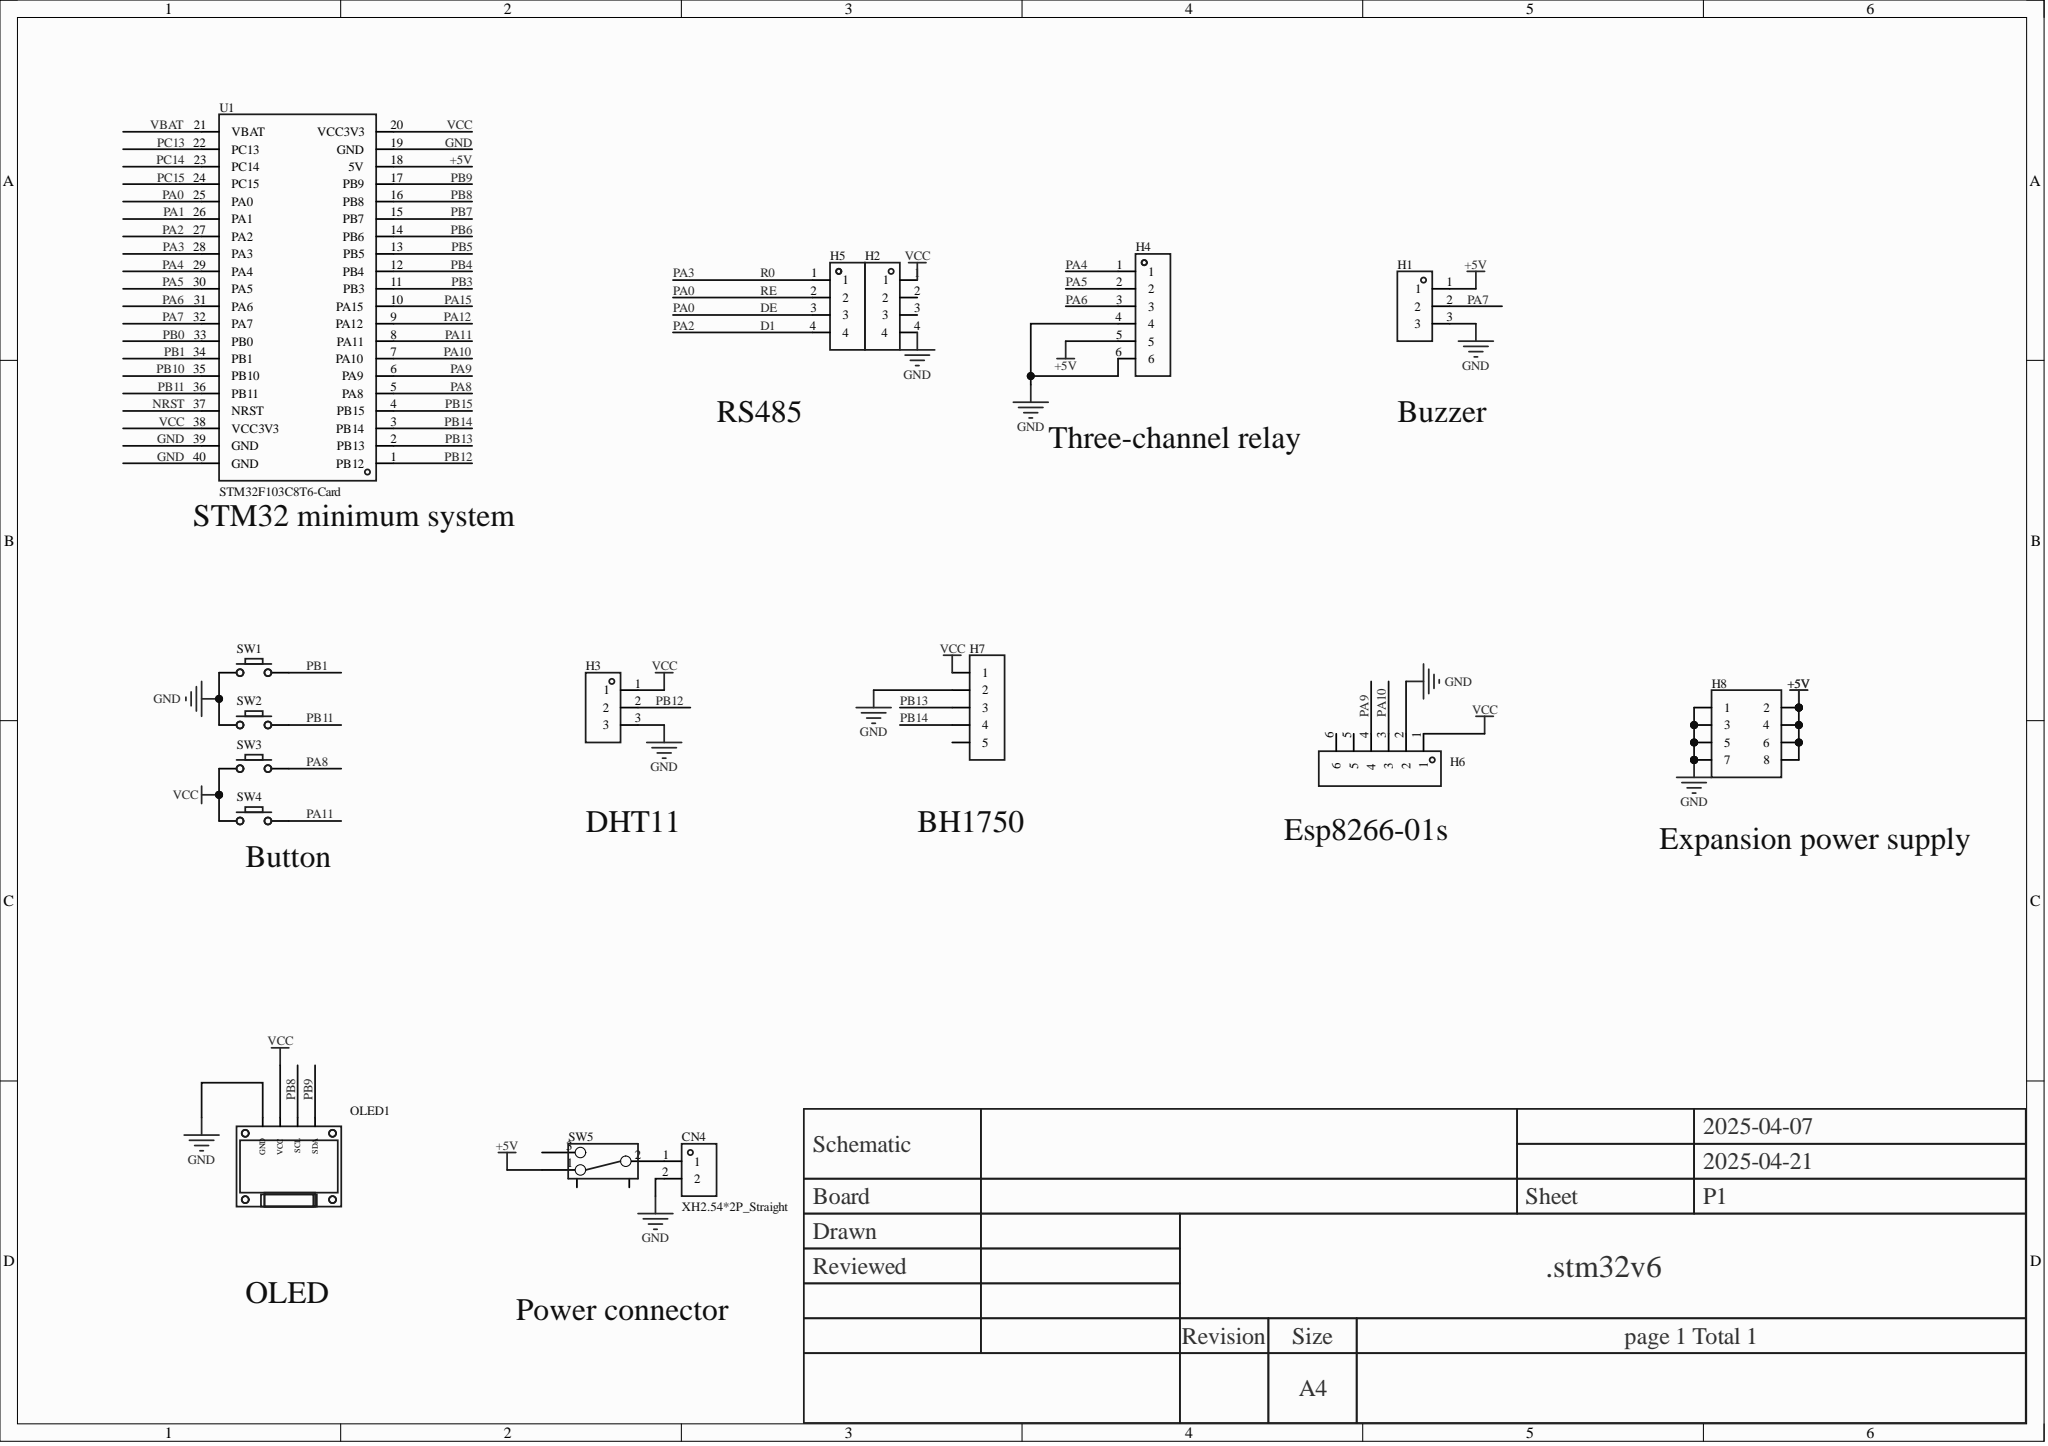Circuit board | Altium Designer | 16 parts | 22 nets
Bill of materials:
Comment,Description,Designator,Footprint,LibRef,Quantity
"XH2.54*2P_Straight","","CN4","CONN-TH_2P-P2.50-XH2.54-2P","XH2.54*2P_直插","1"
"","","H1, H3","HDR-TH_3P-P2.54-V-F","HDR-F_2.54_1x3P","2"
"","","H2, H5","HDR-TH_4P-P2.54-V-F","HDR-F_2.54_1x4P","2"
"","","H4, H6","HDR-TH_6P-P2.54-V-F","HDR-F_2.54_1x6P","2"
"","","H7","HDR-TH_5P-P2.54-V-F","HDR-F_2.54_1x5P","1"
"","","H8","HDR-TH_8P-P2.54-V-F-R2-C4-S2.54-1","HDR-F_2.54_2x4","1"
"","","OLED1","0.96OLED_4P","0.96OLED模块_4P","1"
"","","SW1, SW2, SW3, SW4","Key_TH_3.5x6x4.3","Key_TH_3.5x6x4.3","4"
"","","SW5","拨动开关","拨动开关_正","1"
"STM32F103C8T6-Card","","U1","CONN-TH_L53.3-W22.9_STM32F103C8T6-CARD","STM32F103C8T6-Card","1"
Netlist (Protel format):
[
CN4
CONN-TH_2P-P2.50-XH2.54-2P
XH2.54*2P_Straight



]
[
H1
HDR-TH_3P-P2.54-V-F




]
[
H2
HDR-TH_4P-P2.54-V-F




]
[
H3
HDR-TH_3P-P2.54-V-F




]
[
H4
HDR-TH_6P-P2.54-V-F




]
[
H5
HDR-TH_4P-P2.54-V-F




]
[
H6
HDR-TH_6P-P2.54-V-F




]
[
H7
HDR-TH_5P-P2.54-V-F




]
[
H8
HDR-TH_8P-P2.54-V-F-R2-C4-S2.54-1




]
[
OLED1
0.96OLED_4P




]
[
SW1
Key_TH_3.5x6x4.3




]
[
SW2
Key_TH_3.5x6x4.3




]
[
SW3
Key_TH_3.5x6x4.3




]
[
SW4
Key_TH_3.5x6x4.3




]
[
SW5
拨动开关




]
[
U1
CONN-TH_L53.3-W22.9_STM32F103C8T6-CARD
STM32F103C8T6-Card



]
(
VCC
H2-1
H3-1
H6-1
H7-1
OLED1-2
SW3-A
SW4-A
U1-20
U1-38
)
(
PB14
H7-4
U1-3
)
(
PB13
H7-3
U1-2
)
(
PB12
H3-2
U1-1
)
(
PB11
SW2-B
U1-36
)
(
PB9
OLED1-4
U1-17
)
(
PB8
OLED1-3
U1-16
)
(
PB1
SW1-B
U1-34
)
(
PA11
SW4-B
U1-8
)
(
PA10
H6-3
U1-7
)
(
PA9
H6-4
U1-6
)
(
PA8
SW3-B
U1-5
)
(
PA7
H1-2
U1-32
)
(
PA6
H4-3
U1-31
)
(
PA5
H4-2
U1-30
)
(
PA4
H4-1
U1-29
)
(
PA3
H5-1
U1-28
)
(
NetCN4_1
CN4-1
SW5-2
)
(
GND
CN4-2
H1-3
H2-4
H3-3
H4-4
H4-6
H6-2
H7-2
H8-1
H8-3
H8-5
H8-7
OLED1-1
SW1-A
SW2-A
U1-19
U1-39
U1-40
)
(
DE
H5-2
H5-3
U1-25
)
(
D1
H5-4
U1-27
)
(
+5V
H1-1
H4-5
H8-2
H8-4
H8-6
H8-8
SW5-1
U1-18
)